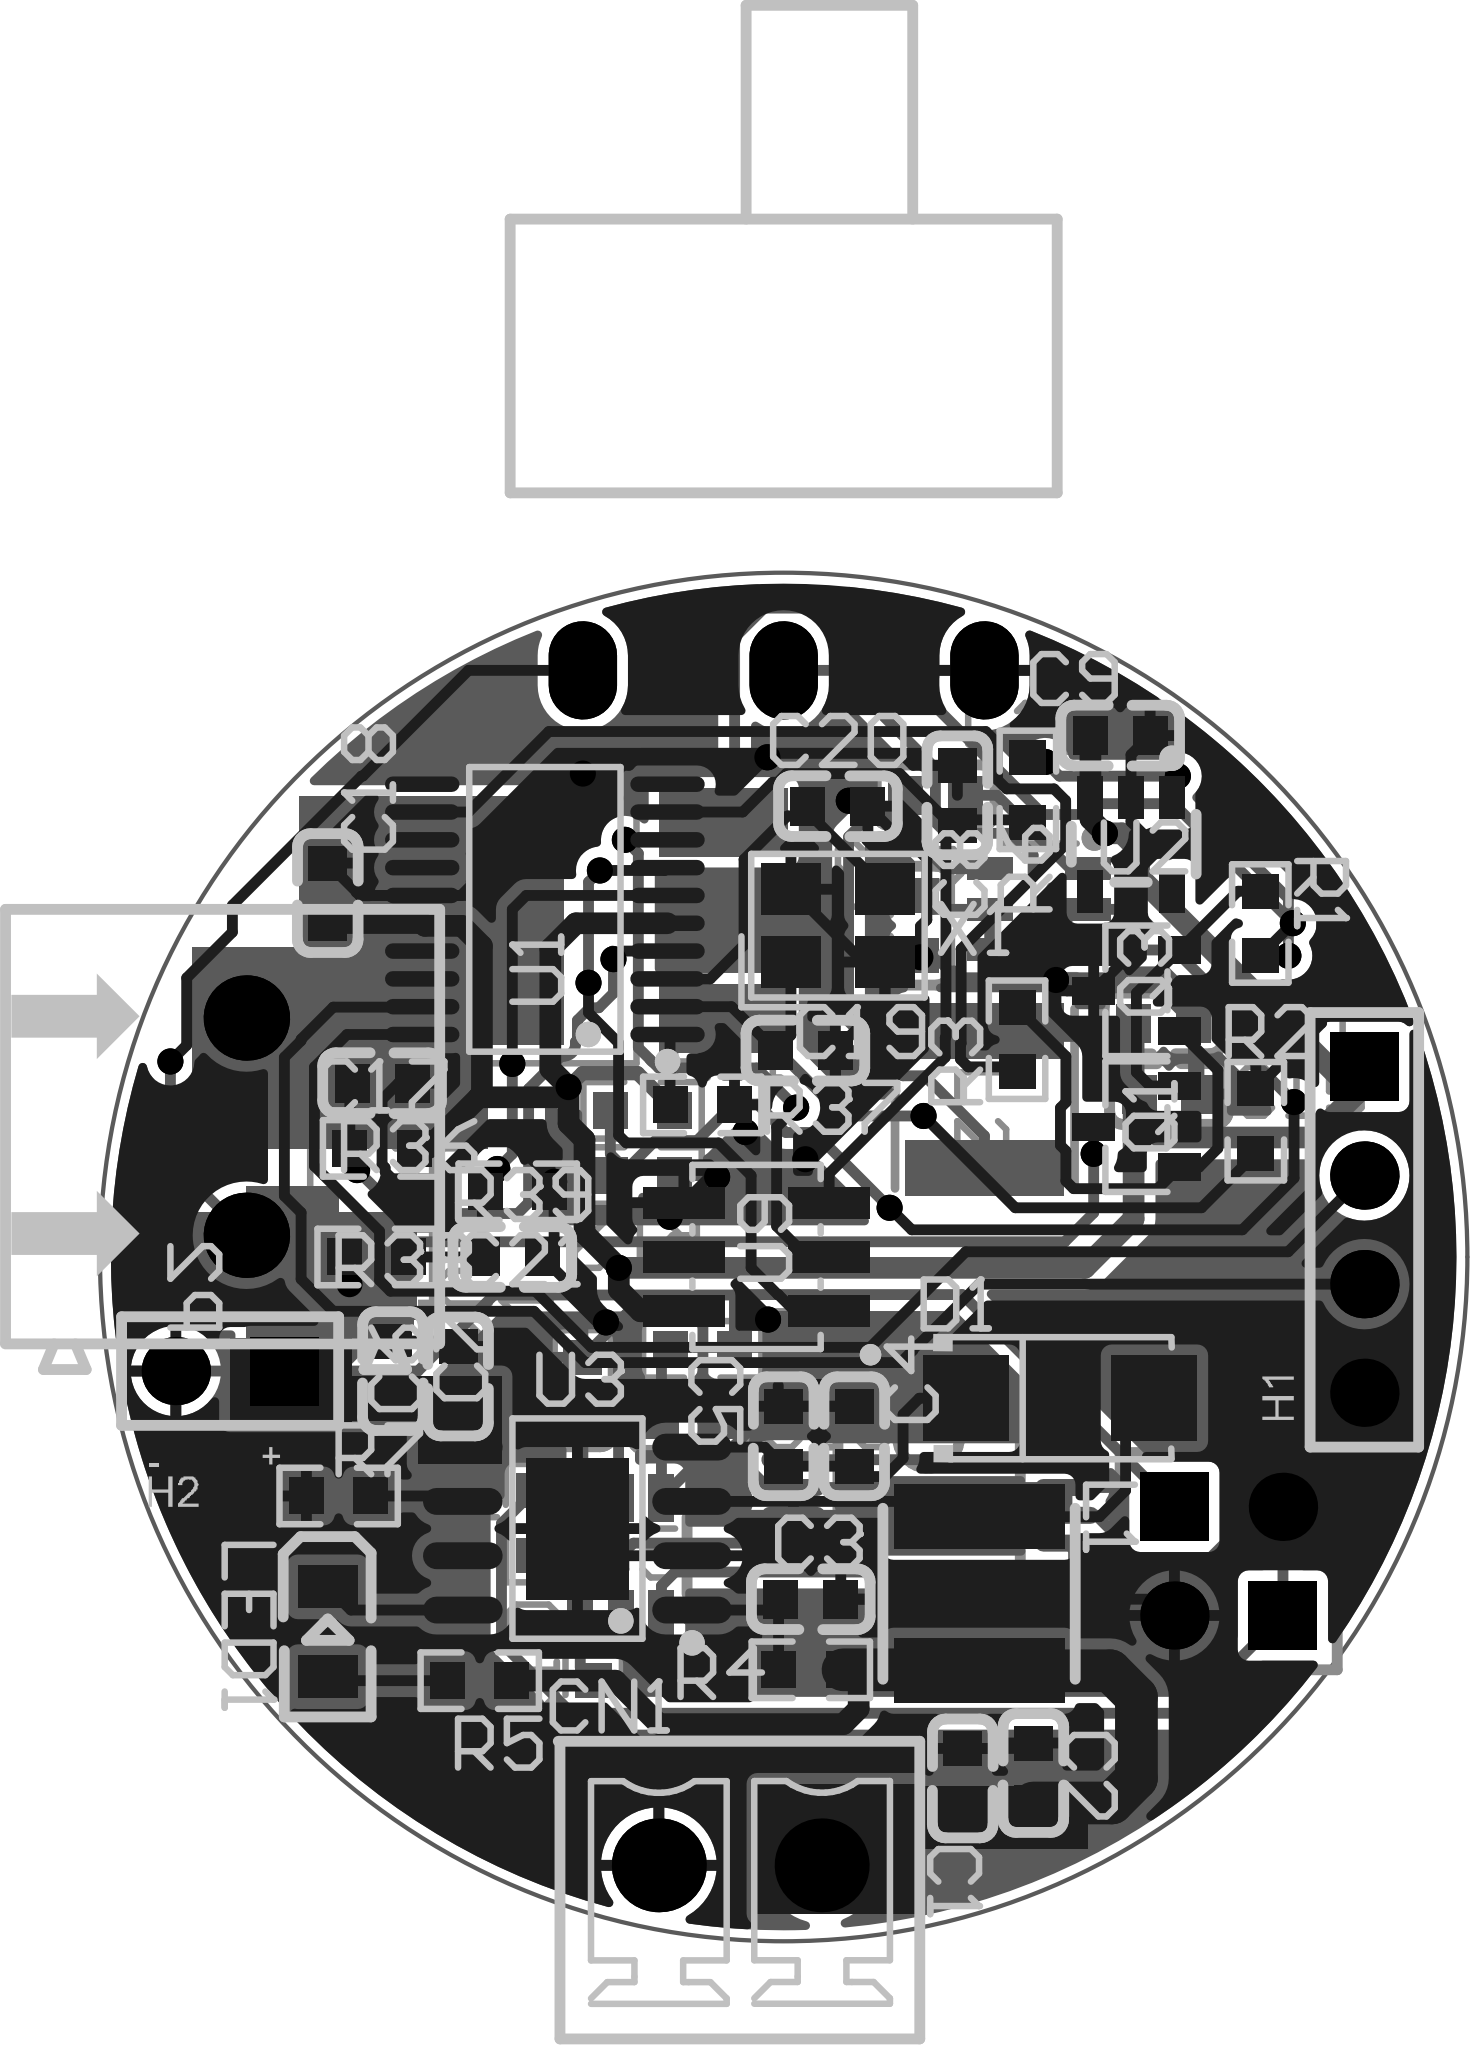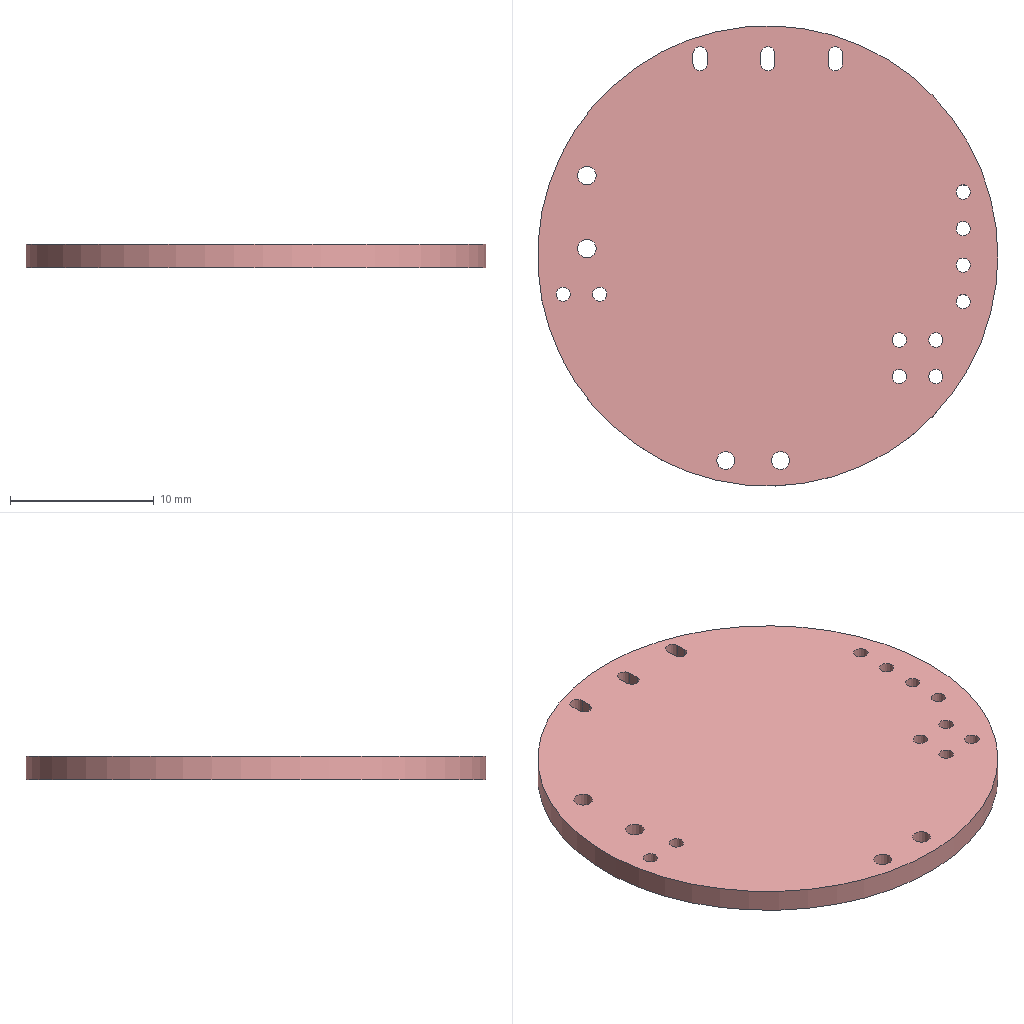Circuit board layout | Altium Designer | box 32 x 32 x 1.6 mm
Layer stack:
# Altium Designer layer stack of  (unit mm; dielectric type: 0 none, 1 core, 2 prepreg, 3 surface material)
index,name,kind,layer,copper_thickness_mm,dielectric_type,dielectric_thickness_mm,dielectric_material,dielectric_constant
0,Top Paste Mask Layer,other,,,,,,
1,Top Silkscreen Layer,other,,,,,,
2,Top Solder Mask Layer,dielectric,,,3,0.0102,,3.3
3,Top Layer,copper,Top Layer,0.0356,,,,
4,Dielectric1,dielectric,,,3,1.509,FR4,4.5
5,Bottom Layer,copper,Bottom Layer,0.0356,,,,
6,Bottom Solder Mask Layer,dielectric,,,3,0.0102,,3.3
7,Bottom Silkscreen Layer,other,,,,,,
8,Bottom Paste Mask Layer,other,,,,,,
# drill layer pairs: low layer,high layer
drill_pair,Top Layer,Bottom Layer
Part placement:
Designator,Comment,Layer,Footprint,Center-X(mm),Center-Y(mm),Rotation
C1,100nF,TopLayer,C0603,102.489,83.058,270
C2,100nF,TopLayer,C0603,104.14,83.185,270
C3,100nF,TopLayer,C0603,98.933,87.249,180
C4,100nF,TopLayer,C0603,99.949,91.059,90
C5,100nF,TopLayer,C0603,98.298,91.059,270
C6,100nF,TopLayer,C0603,89.154,92.583,90
C7,100nF,TopLayer,C0603,90.678,92.456,90
C8,100nF,TopLayer,C0603,102.362,106.045,270
C9,100nF,TopLayer,C0603,106.172,107.442,0
C10,100nF,BottomLayer,C0603,96.139,91.44,180
C11,100nF,BottomLayer,C0603,93.599,92.202,90
C12,100nF,BottomLayer,C0603,101.473,102.997,90
C13,100nF,BottomLayer,C0603,101.854,106.045,0
C14,100nF,BottomLayer,C0603,107.188,100.711,180
C15,100nF,BottomLayer,C0603,107.315,99.06,180
C17,100nF,TopLayer,C0603,88.9,99.314,0
C18,100nF,TopLayer,C0603,87.63,103.759,90
C19,100nF,TopLayer,C0603,98.806,100.076,0
C20,100nF,TopLayer,C0603,99.568,105.791,0
C21,100nF,TopLayer,C0603,91.948,95.25,0
CN1,WJ15EDGVC-3.81-02P-14-00A,TopLayer,CONN-TH_WJ15EDGVC-3.81-2P,97.282,81.026,0
D1,SS34,TopLayer,SMA_L4.3-W2.6-LS5.2-RD,104.775,91.948,0
H1,LAIL-PZ2.54-4P-L,TopLayer,CONN-TH_LAIL-PZ2.54-4P-L,111.887,95.885,270
H3,LAIL-PZ2.54-2P-L,BottomLayer,CONN-TH_LAIL-PZ2.54-2P-L,108.712,89.408,0
H4,LAIL-PZ2.54-2P-L,BottomLayer,CONN-TH_LAIL-PZ2.54-2P-L,108.712,86.868,180
L1,2.2uH,TopLayer,IND-SMD_L4.0-W4.0_LQH44PN2R2MP0L,102.87,87.376,270
L2,4.7uH,BottomLayer,IND-SMD_L4.0-W4.0_SMNR4012,102.997,98.933,90
LED1,KT-0805W,TopLayer,LED0805-R-RD,87.63,86.487,270
P2,WJ500V-5.08-2P,TopLayer,CONN-TH_2P-P5.00_WJ500V-5.08-2P,85.725,98.298,90
Q1,SS8050(RANGE:200-350),TopLayer,SOT-23-3_L2.9-W1.3-P1.90-LS2.4-BR,106.553,98.298,0
Q2,CMD075N06L,BottomLayer,TO-252-2_L6.6-W6.1-P4.57-LS9.9-BR-CW,93.472,103.124,0
Q3,SS8550 Y2(RANGE:200-350),TopLayer,SOT-23-3_L2.9-W1.3-P1.90-LS2.4-BR,106.553,101.473,0
Q4,AP8205A,BottomLayer,TSSOP-8_L4.4-W3.0-P0.65-LS6.4-BL-2,101.727,89.535,270
R1,10K,TopLayer,R0603,109.451,103.048,270
R2,10K,TopLayer,R0603,109.347,98.425,270
R3,10K,TopLayer,R0603,103.759,100.33,90
R4,10K,TopLayer,R0603,98.933,85.598,0
R5,10K,TopLayer,R0603,91.186,85.344,0
R6,10K,TopLayer,R0603,104.013,106.172,90
R7,10K,TopLayer,R0603,87.884,89.662,180
R8,10K,BottomLayer,R0603,92.456,89.027,270
R9,10K,BottomLayer,R0603,96.393,93.091,180
R10,10K,BottomLayer,R0603,93.853,84.582,270
R11,10K,BottomLayer,R0603,94.996,98.679,180
R12,10K,BottomLayer,R0603,94.996,97.155,0
R36,10K,TopLayer,R0603,88.9,97.79,0
R37,10K,TopLayer,R0603,96.393,98.806,0
R38,10K,TopLayer,R0603,88.773,95.25,180
R39,10K,TopLayer,R0603,92.075,96.774,180
U1,GD32E230F8P6TR,TopLayer,TSSOP-20_L6.5-W4.4-P0.65-LS6.4-BL,92.71,103.378,90
U2,SC01T,TopLayer,SOT-23-5_L2.9-W1.6-P0.95-LS2.8-BR,106.426,104.902,90
U3,PW4584A,TopLayer,ESOP-8_L4.9-W3.9-P1.27-LS6.0-BL-EP-1,93.472,88.9,90
U4,SS36,BottomLayer,SMA_L4.3-W2.6-LS5.1-RD,88.646,96.774,90
U5,HY2120-CB,BottomLayer,SOT-23-6_L2.9-W1.6-P0.95-LS2.8-BR,94.488,88.265,270
U6,SS-12D06G5R,TopLayer,SW-TH_SS-12D06G5R,98.298,108.966,180
U7,MT2492,BottomLayer,SOT-23-6_L2.9-W1.6-P0.95-LS2.8-BL_3,104.267,103.378,270
X1,8MHz,TopLayer,CRYSTAL-SMD_4P-L3.2-W2.5-BL,99.568,102.997,0
H2,LAIL-PZ2.54-2P-L,TopLayer,CONN-TH_LAIL-PZ2.54-2P-L,85.344,92.583,180
U9,LAIL-PM1.27-3PX2-T,TopLayer,HDR-SMD_6P-P1.27_LAIL-PM1.27-3PX2-T,97.663,95.25,90
Pad and via stacks:
# Altium Designer via and pad stacks of  (unit mm). Each distinct definition once, with the count of objects using it.
# via: kind,start_layer,end_layer,hole_mm,diameter_mm,mode(0 simple;1 top-mid-bottom;2 full stack),diameter_per_layer,count,example_net
# pad: kind,layer,hole_mm,hole_type(0 round;1 square;2 slot),plating,top_size,top_shape(1 round;2 rect;3 octagon;9 rounded rect),mid_size,bottom_size,mode,footprint,size_per_layer,count,example
pad,Top Layer,0,0,plated,0.8001x0.8992,2,0.8001x0.8992,0.8001x0.8992,0,C0603,,28,C1.2
pad,Top Layer,0,0,plated,1.999x1.999,2,1.999x1.999,1.999x1.999,0,SMA_L4.3-W2.6-LS5.2-RD,,2,D1.2
pad,Top Layer,0,0,plated,1.501x4,2,1.501x4,1.501x4,0,IND-SMD_L4.0-W4.0_LQH44PN2R2MP0L,,2,L1.1
pad,Top Layer,0,0,plated,1.001x1.399,2,1.001x1.399,1.001x1.399,0,LED0805-R-RD,,2,LED1.2
pad,Top Layer,0,0,plated,1.001x0.6502,2,1.001x0.6502,1.001x0.6502,0,SOT-23-3_L2.9-W1.3-P1.90-LS2.4-BR,,6,Q1.1
pad,Top Layer,0,0,plated,0.8077x0.8636,2,0.8077x0.8636,0.8077x0.8636,0,R0603,,22,R1.2
pad,Top Layer,0,0,plated,0.3632x1.742,1,0.3632x1.742,0.3632x1.742,0,TSSOP-20_L6.5-W4.4-P0.65-LS6.4-BL,,20,U1.1
pad,Top Layer,0,0,plated,0.5994x1.001,2,0.5994x1.001,0.5994x1.001,0,SOT-23-5_L2.9-W1.6-P0.95-LS2.8-BR,,5,U2.2
pad,Top Layer,0,0,plated,0.6299x1.864,1,0.6299x1.864,0.6299x1.864,0,ESOP-8_L4.9-W3.9-P1.27-LS6.0-BL-EP-1,,8,U3.5
pad,Top Layer,0,0,plated,3.3x2.4,2,3.3x2.4,3.3x2.4,0,ESOP-8_L4.9-W3.9-P1.27-LS6.0-BL-EP-1,,1,U3.9
pad,Top Layer,0,0,plated,1.399x1.199,2,1.399x1.199,1.399x1.199,0,CRYSTAL-SMD_4P-L3.2-W2.5-BL,,4,X1.1
pad,Top Layer,0,0,plated,0.7391x1.9,2,0.7391x1.9,0.7391x1.9,0,HDR-SMD_6P-P1.27_LAIL-PM1.27-3PX2-T,,6,U9.1
pad,Bottom Layer,0,0,plated,0.8001x0.8992,2,0.8001x0.8992,0.8001x0.8992,0,C0603,,12,C10.2
pad,Bottom Layer,0,0,plated,3.701x1.3,2,3.701x1.3,3.701x1.3,0,IND-SMD_L4.0-W4.0_SMNR4012,,2,L2.2
pad,Bottom Layer,0,0,plated,3x1.6,2,3x1.6,3x1.6,0,TO-252-2_L6.6-W6.1-P4.57-LS9.9-BR-CW,,2,Q2.1
pad,Bottom Layer,0,0,plated,6.2x5.799,2,6.2x5.799,6.2x5.799,0,TO-252-2_L6.6-W6.1-P4.57-LS9.9-BR-CW,,1,Q2.2
pad,Bottom Layer,0,0,plated,0.3988x1.501,1,0.3988x1.501,0.3988x1.501,0,TSSOP-8_L4.4-W3.0-P0.65-LS6.4-BL-2,,8,Q4.1
pad,Bottom Layer,0,0,plated,0.8077x0.8636,2,0.8077x0.8636,0.8077x0.8636,0,R0603,,10,R8.2
pad,Bottom Layer,0,0,plated,1.999x1.999,2,1.999x1.999,1.999x1.999,0,SMA_L4.3-W2.6-LS5.1-RD,,2,U4.1
pad,Bottom Layer,0,0,plated,1.1x0.5994,2,1.1x0.5994,1.1x0.5994,0,SOT-23-6_L2.9-W1.6-P0.95-LS2.8-BR,,6,U5.3
pad,Bottom Layer,0,0,plated,0.5309x1.072,2,0.5309x1.072,0.5309x1.072,0,SOT-23-6_L2.9-W1.6-P0.95-LS2.8-BL_3,,6,U7.6
pad,Multi-Layer,1.25,0,plated,2.2x2.2,1,2.2x2.2,2.2x2.2,0,CONN-TH_WJ15EDGVC-3.81-2P,,2,CN1.1
pad,Multi-Layer,1.001,0,plated,1.6x1.6,2,1.6x1.6,1.6x1.6,0,CONN-TH_LAIL-PZ2.54-4P-L,,1,H1.1
pad,Multi-Layer,1.001,0,plated,1.6x1.6,1,1.6x1.6,1.6x1.6,0,CONN-TH_LAIL-PZ2.54-4P-L,,3,H1.2
pad,Multi-Layer,1.001,0,plated,1.6x1.6,1,1.6x1.6,1.6x1.6,0,CONN-TH_LAIL-PZ2.54-2P-L,,3,H3.2
pad,Multi-Layer,1.001,0,plated,1.6x1.6,2,1.6x1.6,1.6x1.6,0,CONN-TH_LAIL-PZ2.54-2P-L,,3,H3.1
pad,Multi-Layer,1.3,0,plated,1.999x1.999,1,1.999x1.999,1.999x1.999,0,CONN-TH_2P-P5.00_WJ500V-5.08-2P,,2,P2.2
pad,Multi-Layer,1.001,2,plated,1.6x2.301,1,1.6x2.301,1.6x2.301,0,SW-TH_SS-12D06G5R,,3,U6.3
via,Top Layer,Bottom Layer,0.3048,0.6096,0,,33,$1N7
Copper pours:
name,layer,net,type(0 solid;1 hatched;2 none)
Bottom Layer-GND,Bottom Layer,GND,0
Top Layer-GND,Top Layer,GND,0
Design rules, without the lines most boards share:
# Altium Designer design rules of  (exported by Altium Designer, unit mm)
# columns: name | kind | enabled | priority | scope1 | scope2 | descriptor | typed fields (field=value)
HoleToHoleClearance | 52 | enabled | 1 | All | All | Hole To Hole Clearance (Gap=10mil) (All),(All) | gap=0.254
copperThickness1oz | 0 | enabled | 1 | All | All | Clearance Constraint (Gap=7mil) (All),(All) | gap=0.1778
copperThickness1oz_1 | 63 | enabled | 1 | All | All | Board Clearance Constraint (Gap=0mil) (All) |
copperThickness2oz | 0 | enabled | 2 | All | All | Clearance Constraint (Gap=7mil) (All),(All) | gap=0.1778
copperThickness2oz_1 | 63 | enabled | 2 | All | All | Board Clearance Constraint (Gap=0mil) (All) |
otherClearance | 0 | enabled | 3 | All | All | Clearance Constraint (Gap=7mil) (All),(All) | gap=0.1778
otherClearance_1 | 63 | enabled | 3 | All | All | Board Clearance Constraint (Gap=0mil) (All) |
copperThickness1oz_2 | 2 | enabled | 1 | All | All | Width Constraint (Min=5mil) (Max=100mil) (Preferred=10mil) (All) |
copperThickness2oz_2 | 2 | enabled | 2 | All | All | Width Constraint (Min=8mil) (Max=100mil) (Preferred=20mil) (All) |
viaSize | 11 | enabled | 1 | All | All | Routing Via (MinHoleWidth=11.811mil) (MaxHoleWidth=248.031mil) (PreferredHoleWidth=12.008mil) (MinWidth=11.811mil) (MaxWidth=248.031mil) (PreferedWidth=12.008mil) (All) | via_min_hole=0.3 via_max_hole=6.3 via_preferred_diameter=0.305 via_preferred_hole=0.305